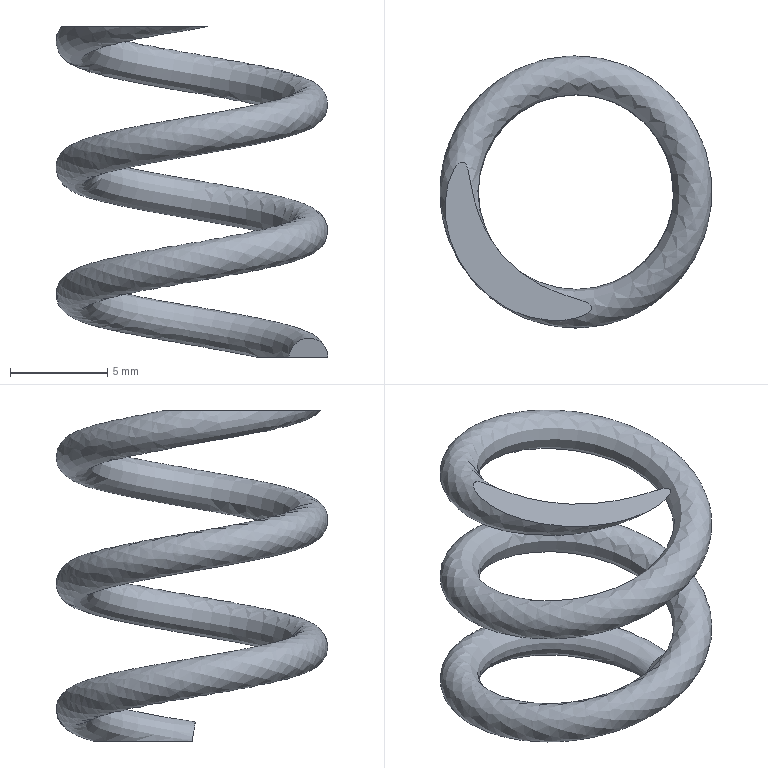Part | NX | features DATUM_CSYS 2, SKETCH 2, DATUM_ON_PATH 1, EXTRUDE 1, HELIX 1, SKIN 1 | 1 solid | 4 faces | box 13.997 x 13.994 x 17 mm | volume 306.817 mm3 | plane 3 | spline 1